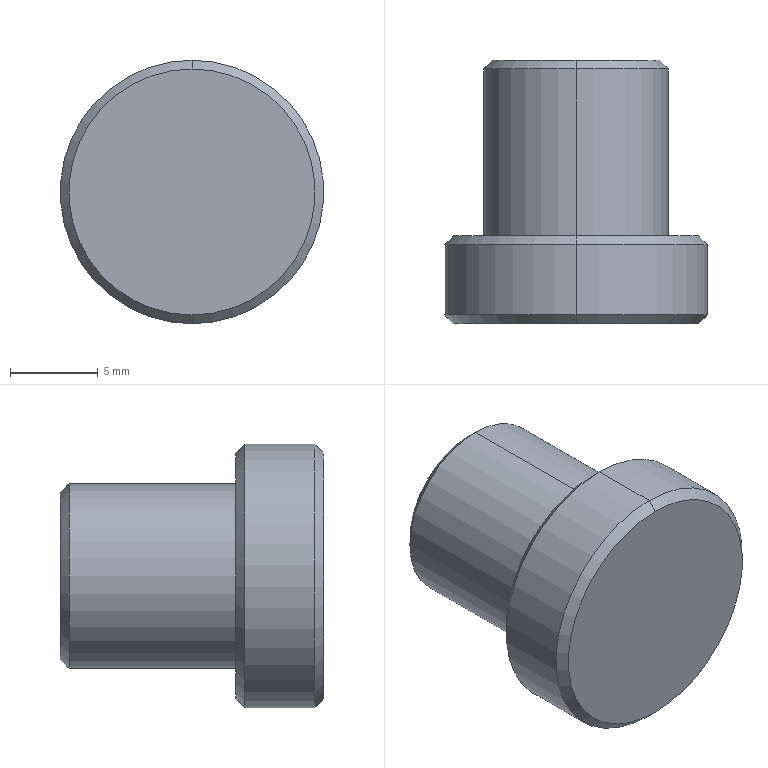Part | SolidWorks | features Chamfer 1, Revolution 1 | 1 solid | 13 faces | box 15 x 15 x 15 mm | volume 1734 mm3 | cone 6 | cylinder 4 | plane 3 | commonest cylinder face diameters 10.5 x2 15 x2
STEP:
#1=CARTESIAN_POINT('',(0.,15.,4.75));
#2=VERTEX_POINT('',#1);
#3=CARTESIAN_POINT('',(0.,15.,-4.75));
#4=VERTEX_POINT('',#3);
#5=CARTESIAN_POINT('',(0.,15.,0.));
#6=DIRECTION('',(0.,1.,0.));
#7=DIRECTION('',(0.,0.,1.));
#8=AXIS2_PLACEMENT_3D('',#5,#6,#7);
#9=CIRCLE('',#8,4.75);
#10=EDGE_CURVE('',#2,#4,#9,.T.);
#11=ORIENTED_EDGE('',*,*,#10,.F.);
#12=CARTESIAN_POINT('',(0.,14.5,5.25));
#13=VERTEX_POINT('',#12);
#14=CARTESIAN_POINT('',(0.,14.5,5.25));
#15=DIRECTION('',(0.,-0.7071,0.7071));
#16=VECTOR('',#15,1000.);
#17=LINE('',#14,#16);
#18=EDGE_CURVE('',#2,#13,#17,.T.);
#19=ORIENTED_EDGE('',*,*,#18,.T.);
#20=CARTESIAN_POINT('',(0.,14.5,-5.25));
#21=VERTEX_POINT('',#20);
#22=CARTESIAN_POINT('',(0.,14.5,0.));
#23=DIRECTION('',(0.,-1.,0.));
#24=DIRECTION('',(0.,0.,1.));
#25=AXIS2_PLACEMENT_3D('',#22,#23,#24);
#26=CIRCLE('',#25,5.25);
#27=EDGE_CURVE('',#21,#13,#26,.T.);
#28=ORIENTED_EDGE('',*,*,#27,.F.);
#29=CARTESIAN_POINT('',(0.,14.5,-5.25));
#30=DIRECTION('',(0.,-0.7071,-0.7071));
#31=VECTOR('',#30,1000.);
#32=LINE('',#29,#31);
#33=EDGE_CURVE('',#4,#21,#32,.T.);
#34=ORIENTED_EDGE('',*,*,#33,.F.);
#35=EDGE_LOOP('',(#11,#19,#28,#34));
#36=FACE_OUTER_BOUND('',#35,.T.);
#37=CARTESIAN_POINT('',(0.,14.5,0.));
#38=DIRECTION('',(0.,-1.,0.));
#39=DIRECTION('',(0.,0.,-1.));
#40=AXIS2_PLACEMENT_3D('',#37,#38,#39);
#41=CONICAL_SURFACE('',#40,5.25,0.7854);
#42=ADVANCED_FACE('',(#36),#41,.T.);
#43=CARTESIAN_POINT('',(0.,5.,7.));
#44=VERTEX_POINT('',#43);
#45=CARTESIAN_POINT('',(0.,5.,-7.));
#46=VERTEX_POINT('',#45);
#47=CARTESIAN_POINT('',(0.,5.,0.));
#48=DIRECTION('',(0.,1.,0.));
#49=DIRECTION('',(0.,0.,1.));
#50=AXIS2_PLACEMENT_3D('',#47,#48,#49);
#51=CIRCLE('',#50,7.);
#52=EDGE_CURVE('',#44,#46,#51,.T.);
#53=ORIENTED_EDGE('',*,*,#52,.F.);
#54=CARTESIAN_POINT('',(0.,4.5,7.5));
#55=VERTEX_POINT('',#54);
#56=CARTESIAN_POINT('',(0.,4.5,7.5));
#57=DIRECTION('',(0.,-0.7071,0.7071));
#58=VECTOR('',#57,1000.);
#59=LINE('',#56,#58);
#60=EDGE_CURVE('',#44,#55,#59,.T.);
#61=ORIENTED_EDGE('',*,*,#60,.T.);
#62=CARTESIAN_POINT('',(0.,4.5,-7.5));
#63=VERTEX_POINT('',#62);
#64=CARTESIAN_POINT('',(0.,4.5,0.));
#65=DIRECTION('',(0.,-1.,0.));
#66=DIRECTION('',(0.,0.,1.));
#67=AXIS2_PLACEMENT_3D('',#64,#65,#66);
#68=CIRCLE('',#67,7.5);
#69=EDGE_CURVE('',#63,#55,#68,.T.);
#70=ORIENTED_EDGE('',*,*,#69,.F.);
#71=CARTESIAN_POINT('',(0.,4.5,-7.5));
#72=DIRECTION('',(0.,-0.7071,-0.7071));
#73=VECTOR('',#72,1000.);
#74=LINE('',#71,#73);
#75=EDGE_CURVE('',#46,#63,#74,.T.);
#76=ORIENTED_EDGE('',*,*,#75,.F.);
#77=EDGE_LOOP('',(#53,#61,#70,#76));
#78=FACE_OUTER_BOUND('',#77,.T.);
#79=CARTESIAN_POINT('',(0.,4.5,0.));
#80=DIRECTION('',(0.,-1.,0.));
#81=DIRECTION('',(0.,0.,-1.));
#82=AXIS2_PLACEMENT_3D('',#79,#80,#81);
#83=CONICAL_SURFACE('',#82,7.5,0.7854);
#84=ADVANCED_FACE('',(#78),#83,.T.);
#85=CARTESIAN_POINT('',(0.,0.,-7.));
#86=VERTEX_POINT('',#85);
#87=CARTESIAN_POINT('',(0.,0.,7.));
#88=VERTEX_POINT('',#87);
#89=CARTESIAN_POINT('',(0.,0.,0.));
#90=DIRECTION('',(0.,-1.,0.));
#91=DIRECTION('',(0.,0.,-1.));
#92=AXIS2_PLACEMENT_3D('',#89,#90,#91);
#93=CIRCLE('',#92,7.);
#94=EDGE_CURVE('',#86,#88,#93,.T.);
#95=ORIENTED_EDGE('',*,*,#94,.F.);
#96=CARTESIAN_POINT('',(0.,0.5,-7.5));
#97=VERTEX_POINT('',#96);
#98=CARTESIAN_POINT('',(0.,0.,-7.));
#99=DIRECTION('',(0.,0.7071,-0.7071));
#100=VECTOR('',#99,1000.);
#101=LINE('',#98,#100);
#102=EDGE_CURVE('',#86,#97,#101,.T.);
#103=ORIENTED_EDGE('',*,*,#102,.T.);
#104=CARTESIAN_POINT('',(0.,0.5,7.5));
#105=VERTEX_POINT('',#104);
#106=CARTESIAN_POINT('',(0.,0.5,0.));
#107=DIRECTION('',(0.,1.,0.));
#108=DIRECTION('',(0.,0.,-1.));
#109=AXIS2_PLACEMENT_3D('',#106,#107,#108);
#110=CIRCLE('',#109,7.5);
#111=EDGE_CURVE('',#105,#97,#110,.T.);
#112=ORIENTED_EDGE('',*,*,#111,.F.);
#113=CARTESIAN_POINT('',(0.,0.,7.));
#114=DIRECTION('',(0.,0.7071,0.7071));
#115=VECTOR('',#114,1000.);
#116=LINE('',#113,#115);
#117=EDGE_CURVE('',#88,#105,#116,.T.);
#118=ORIENTED_EDGE('',*,*,#117,.F.);
#119=EDGE_LOOP('',(#95,#103,#112,#118));
#120=FACE_OUTER_BOUND('',#119,.T.);
#121=CARTESIAN_POINT('',(0.,0.,0.));
#122=DIRECTION('',(0.,1.,0.));
#123=DIRECTION('',(0.,0.,1.));
#124=AXIS2_PLACEMENT_3D('',#121,#122,#123);
#125=CONICAL_SURFACE('',#124,7.,0.7854);
#126=ADVANCED_FACE('',(#120),#125,.T.);
#127=ORIENTED_EDGE('',*,*,#69,.T.);
#128=CARTESIAN_POINT('',(0.,0.,7.5));
#129=DIRECTION('',(0.,-1.,0.));
#130=VECTOR('',#129,1000.);
#131=LINE('',#128,#130);
#132=EDGE_CURVE('',#55,#105,#131,.T.);
#133=ORIENTED_EDGE('',*,*,#132,.T.);
#134=ORIENTED_EDGE('',*,*,#111,.T.);
#135=CARTESIAN_POINT('',(0.,0.,-7.5));
#136=DIRECTION('',(0.,-1.,0.));
#137=VECTOR('',#136,1000.);
#138=LINE('',#135,#137);
#139=EDGE_CURVE('',#63,#97,#138,.T.);
#140=ORIENTED_EDGE('',*,*,#139,.F.);
#141=EDGE_LOOP('',(#127,#133,#134,#140));
#142=FACE_OUTER_BOUND('',#141,.T.);
#143=CARTESIAN_POINT('',(0.,0.,0.));
#144=DIRECTION('',(0.,-1.,0.));
#145=DIRECTION('',(0.,0.,-1.));
#146=AXIS2_PLACEMENT_3D('',#143,#144,#145);
#147=CYLINDRICAL_SURFACE('',#146,7.5);
#148=ADVANCED_FACE('',(#142),#147,.T.);
#149=ORIENTED_EDGE('',*,*,#27,.T.);
#150=CARTESIAN_POINT('',(0.,5.,5.25));
#151=VERTEX_POINT('',#150);
#152=CARTESIAN_POINT('',(0.,0.,5.25));
#153=DIRECTION('',(0.,-1.,0.));
#154=VECTOR('',#153,1000.);
#155=LINE('',#152,#154);
#156=EDGE_CURVE('',#13,#151,#155,.T.);
#157=ORIENTED_EDGE('',*,*,#156,.T.);
#158=CARTESIAN_POINT('',(0.,5.,-5.25));
#159=VERTEX_POINT('',#158);
#160=CARTESIAN_POINT('',(0.,5.,0.));
#161=DIRECTION('',(0.,-1.,0.));
#162=DIRECTION('',(0.,0.,-1.));
#163=AXIS2_PLACEMENT_3D('',#160,#161,#162);
#164=CIRCLE('',#163,5.25);
#165=EDGE_CURVE('',#159,#151,#164,.T.);
#166=ORIENTED_EDGE('',*,*,#165,.F.);
#167=CARTESIAN_POINT('',(0.,0.,-5.25));
#168=DIRECTION('',(0.,-1.,0.));
#169=VECTOR('',#168,1000.);
#170=LINE('',#167,#169);
#171=EDGE_CURVE('',#21,#159,#170,.T.);
#172=ORIENTED_EDGE('',*,*,#171,.F.);
#173=EDGE_LOOP('',(#149,#157,#166,#172));
#174=FACE_OUTER_BOUND('',#173,.T.);
#175=CARTESIAN_POINT('',(0.,0.,0.));
#176=DIRECTION('',(0.,-1.,0.));
#177=DIRECTION('',(0.,0.,-1.));
#178=AXIS2_PLACEMENT_3D('',#175,#176,#177);
#179=CYLINDRICAL_SURFACE('',#178,5.25);
#180=ADVANCED_FACE('',(#174),#179,.T.);
#181=CARTESIAN_POINT('',(0.,15.,0.));
#182=DIRECTION('',(0.,1.,0.));
#183=DIRECTION('',(0.,0.,1.));
#184=AXIS2_PLACEMENT_3D('',#181,#182,#183);
#185=CIRCLE('',#184,4.75);
#186=EDGE_CURVE('',#4,#2,#185,.T.);
#187=ORIENTED_EDGE('',*,*,#186,.T.);
#188=ORIENTED_EDGE('',*,*,#10,.T.);
#189=EDGE_LOOP('',(#187,#188));
#190=FACE_OUTER_BOUND('',#189,.T.);
#191=CARTESIAN_POINT('',(0.,15.,0.));
#192=DIRECTION('',(0.,1.,0.));
#193=DIRECTION('',(0.,0.,1.));
#194=AXIS2_PLACEMENT_3D('',#191,#192,#193);
#195=PLANE('',#194);
#196=ADVANCED_FACE('',(#190),#195,.T.);
#197=ORIENTED_EDGE('',*,*,#156,.F.);
#198=CARTESIAN_POINT('',(0.,14.5,0.));
#199=DIRECTION('',(0.,-1.,0.));
#200=DIRECTION('',(0.,0.,1.));
#201=AXIS2_PLACEMENT_3D('',#198,#199,#200);
#202=CIRCLE('',#201,5.25);
#203=EDGE_CURVE('',#13,#21,#202,.T.);
#204=ORIENTED_EDGE('',*,*,#203,.T.);
#205=ORIENTED_EDGE('',*,*,#171,.T.);
#206=CARTESIAN_POINT('',(0.,5.,0.));
#207=DIRECTION('',(0.,-1.,0.));
#208=DIRECTION('',(0.,0.,-1.));
#209=AXIS2_PLACEMENT_3D('',#206,#207,#208);
#210=CIRCLE('',#209,5.25);
#211=EDGE_CURVE('',#151,#159,#210,.T.);
#212=ORIENTED_EDGE('',*,*,#211,.F.);
#213=EDGE_LOOP('',(#197,#204,#205,#212));
#214=FACE_OUTER_BOUND('',#213,.T.);
#215=CARTESIAN_POINT('',(0.,0.,0.));
#216=DIRECTION('',(0.,-1.,0.));
#217=DIRECTION('',(0.,0.,-1.));
#218=AXIS2_PLACEMENT_3D('',#215,#216,#217);
#219=CYLINDRICAL_SURFACE('',#218,5.25);
#220=ADVANCED_FACE('',(#214),#219,.T.);
#221=CARTESIAN_POINT('',(0.,5.,0.));
#222=DIRECTION('',(0.,1.,0.));
#223=DIRECTION('',(0.,0.,1.));
#224=AXIS2_PLACEMENT_3D('',#221,#222,#223);
#225=CIRCLE('',#224,7.);
#226=EDGE_CURVE('',#46,#44,#225,.T.);
#227=ORIENTED_EDGE('',*,*,#226,.T.);
#228=ORIENTED_EDGE('',*,*,#52,.T.);
#229=EDGE_LOOP('',(#227,#228));
#230=FACE_OUTER_BOUND('',#229,.T.);
#231=ORIENTED_EDGE('',*,*,#165,.T.);
#232=ORIENTED_EDGE('',*,*,#211,.T.);
#233=EDGE_LOOP('',(#231,#232));
#234=FACE_BOUND('',#233,.T.);
#235=CARTESIAN_POINT('',(0.,5.,-5.25));
#236=DIRECTION('',(0.,1.,0.));
#237=DIRECTION('',(0.,0.,1.));
#238=AXIS2_PLACEMENT_3D('',#235,#236,#237);
#239=PLANE('',#238);
#240=ADVANCED_FACE('',(#230,#234),#239,.T.);
#241=ORIENTED_EDGE('',*,*,#132,.F.);
#242=CARTESIAN_POINT('',(0.,4.5,0.));
#243=DIRECTION('',(0.,-1.,0.));
#244=DIRECTION('',(0.,0.,1.));
#245=AXIS2_PLACEMENT_3D('',#242,#243,#244);
#246=CIRCLE('',#245,7.5);
#247=EDGE_CURVE('',#55,#63,#246,.T.);
#248=ORIENTED_EDGE('',*,*,#247,.T.);
#249=ORIENTED_EDGE('',*,*,#139,.T.);
#250=CARTESIAN_POINT('',(0.,0.5,0.));
#251=DIRECTION('',(0.,1.,0.));
#252=DIRECTION('',(0.,0.,-1.));
#253=AXIS2_PLACEMENT_3D('',#250,#251,#252);
#254=CIRCLE('',#253,7.5);
#255=EDGE_CURVE('',#97,#105,#254,.T.);
#256=ORIENTED_EDGE('',*,*,#255,.T.);
#257=EDGE_LOOP('',(#241,#248,#249,#256));
#258=FACE_OUTER_BOUND('',#257,.T.);
#259=CARTESIAN_POINT('',(0.,0.,0.));
#260=DIRECTION('',(0.,-1.,0.));
#261=DIRECTION('',(0.,0.,-1.));
#262=AXIS2_PLACEMENT_3D('',#259,#260,#261);
#263=CYLINDRICAL_SURFACE('',#262,7.5);
#264=ADVANCED_FACE('',(#258),#263,.T.);
#265=CARTESIAN_POINT('',(0.,0.,0.));
#266=DIRECTION('',(0.,-1.,0.));
#267=DIRECTION('',(0.,0.,-1.));
#268=AXIS2_PLACEMENT_3D('',#265,#266,#267);
#269=CIRCLE('',#268,7.);
#270=EDGE_CURVE('',#88,#86,#269,.T.);
#271=ORIENTED_EDGE('',*,*,#270,.T.);
#272=ORIENTED_EDGE('',*,*,#94,.T.);
#273=EDGE_LOOP('',(#271,#272));
#274=FACE_OUTER_BOUND('',#273,.T.);
#275=CARTESIAN_POINT('',(0.,0.,-7.5));
#276=DIRECTION('',(0.,-1.,0.));
#277=DIRECTION('',(0.,0.,-1.));
#278=AXIS2_PLACEMENT_3D('',#275,#276,#277);
#279=PLANE('',#278);
#280=ADVANCED_FACE('',(#274),#279,.T.);
#281=ORIENTED_EDGE('',*,*,#102,.F.);
#282=ORIENTED_EDGE('',*,*,#270,.F.);
#283=ORIENTED_EDGE('',*,*,#117,.T.);
#284=ORIENTED_EDGE('',*,*,#255,.F.);
#285=EDGE_LOOP('',(#281,#282,#283,#284));
#286=FACE_OUTER_BOUND('',#285,.T.);
#287=CARTESIAN_POINT('',(0.,0.,0.));
#288=DIRECTION('',(0.,1.,0.));
#289=DIRECTION('',(0.,0.,1.));
#290=AXIS2_PLACEMENT_3D('',#287,#288,#289);
#291=CONICAL_SURFACE('',#290,7.,0.7854);
#292=ADVANCED_FACE('',(#286),#291,.T.);
#293=ORIENTED_EDGE('',*,*,#60,.F.);
#294=ORIENTED_EDGE('',*,*,#226,.F.);
#295=ORIENTED_EDGE('',*,*,#75,.T.);
#296=ORIENTED_EDGE('',*,*,#247,.F.);
#297=EDGE_LOOP('',(#293,#294,#295,#296));
#298=FACE_OUTER_BOUND('',#297,.T.);
#299=CARTESIAN_POINT('',(0.,4.5,0.));
#300=DIRECTION('',(0.,-1.,0.));
#301=DIRECTION('',(0.,0.,-1.));
#302=AXIS2_PLACEMENT_3D('',#299,#300,#301);
#303=CONICAL_SURFACE('',#302,7.5,0.7854);
#304=ADVANCED_FACE('',(#298),#303,.T.);
#305=ORIENTED_EDGE('',*,*,#18,.F.);
#306=ORIENTED_EDGE('',*,*,#186,.F.);
#307=ORIENTED_EDGE('',*,*,#33,.T.);
#308=ORIENTED_EDGE('',*,*,#203,.F.);
#309=EDGE_LOOP('',(#305,#306,#307,#308));
#310=FACE_OUTER_BOUND('',#309,.T.);
#311=CARTESIAN_POINT('',(0.,14.5,0.));
#312=DIRECTION('',(0.,-1.,0.));
#313=DIRECTION('',(0.,0.,-1.));
#314=AXIS2_PLACEMENT_3D('',#311,#312,#313);
#315=CONICAL_SURFACE('',#314,5.25,0.7854);
#316=ADVANCED_FACE('',(#310),#315,.T.);
#317=CLOSED_SHELL('',(#42,#84,#126,#148,#180,#196,#220,#240,#264,#280,#292,#304,#316));
#318=MANIFOLD_SOLID_BREP('',#317);
#319=CARTESIAN_POINT('',(0.,0.,0.));
#320=DIRECTION('',(0.,0.,1.));
#321=DIRECTION('',(1.,0.,0.));
#322=AXIS2_PLACEMENT_3D('',#319,#320,#321);
#323=(LENGTH_UNIT()NAMED_UNIT(*)SI_UNIT(.MILLI.,.METRE.));
#324=UNCERTAINTY_MEASURE_WITH_UNIT(LENGTH_MEASURE(0.00001),#323,'','');
#325=(NAMED_UNIT(*)PLANE_ANGLE_UNIT()SI_UNIT($,.RADIAN.));
#326=(NAMED_UNIT(*)SI_UNIT($,.STERADIAN.)SOLID_ANGLE_UNIT());
#327=(GEOMETRIC_REPRESENTATION_CONTEXT(3)GLOBAL_UNCERTAINTY_ASSIGNED_CONTEXT((#324))GLOBAL_UNIT_ASSIGNED_CONTEXT((#323,#325,#326))REPRESENTATION_CONTEXT('',''));
#328=ADVANCED_BREP_SHAPE_REPRESENTATION('',(#318,#322),#327);